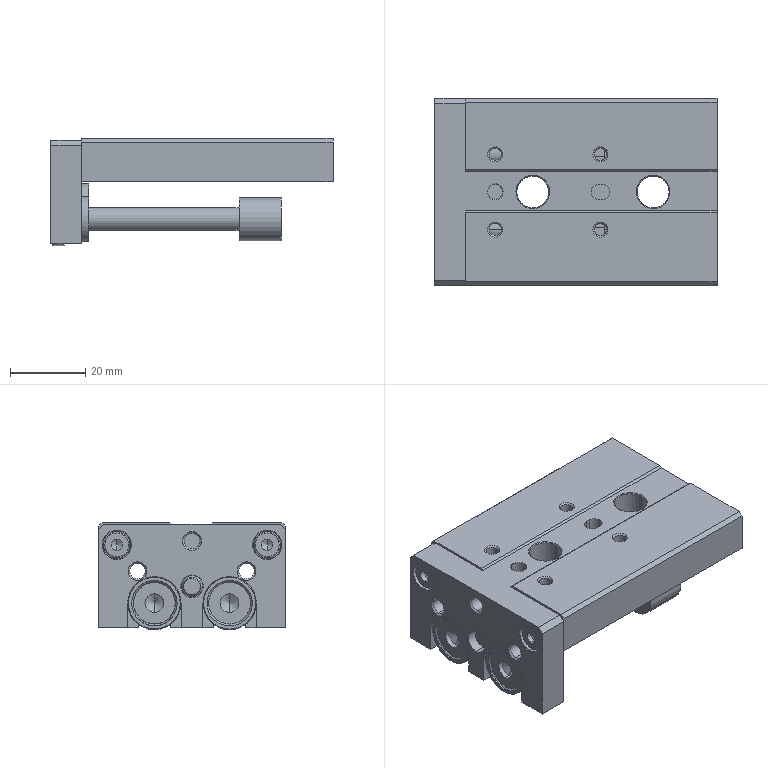Part | SolidWorks | features BaseBody 1 | 1 solid | 253 faces | box 75 x 49.9 x 28.55 mm | volume 42408 mm3 | plane 106 | cylinder 95 | cone 46 | spline 6 | commonest cylinder face diameters 3.242 x12 7.5 x8 8.5 x8 4.134 x6 5 x6 6 x6